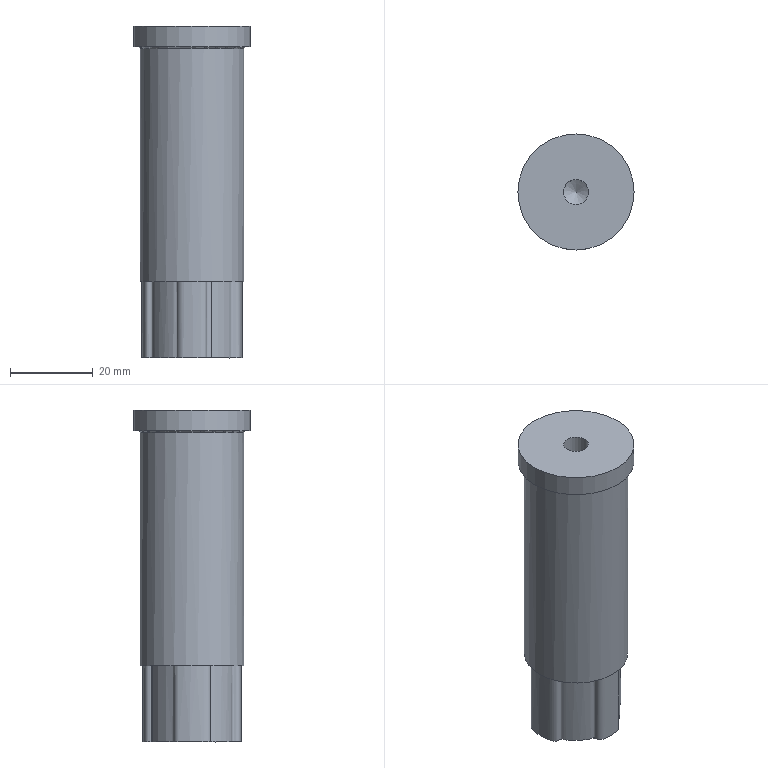Part | NX | features solid 2 | 1 solid | 12 faces | box 28 x 28 x 80 mm | volume 38145 mm3 | plane 4 | cylinder 3 | spline 3 | torus 1 | cone 1 | commonest cylinder face diameters 6 x1 25 x1 28 x1
STEP:
#1=CARTESIAN_POINT('',(12.5,-553.396,-52.641));
#2=VERTEX_POINT('',#1);
#3=CARTESIAN_POINT('',(0.,-553.396,-52.641));
#4=DIRECTION('',(0.,0.,1.));
#5=DIRECTION('',(1.,0.,0.));
#6=AXIS2_PLACEMENT_3D('',#3,#4,#5);
#7=CIRCLE('',#6,12.5);
#8=EDGE_CURVE('',#2,#2,#7,.T.);
#9=ORIENTED_EDGE('',*,*,#8,.F.);
#10=EDGE_LOOP('',(#9));
#11=FACE_BOUND('',#10,.T.);
#12=CARTESIAN_POINT('',(-4.603,-543.997,-52.641));
#13=VERTEX_POINT('',#12);
#14=CARTESIAN_POINT('',(-4.513,-543.694,-52.641));
#15=VERTEX_POINT('',#14);
#16=CARTESIAN_POINT('',(-4.513,-543.694,-52.641));
#17=CARTESIAN_POINT('',(-4.512,-543.806,-52.641));
#18=CARTESIAN_POINT('',(-4.502,-543.949,-52.641));
#19=CARTESIAN_POINT('',(-4.603,-543.997,-52.641));
#20=B_SPLINE_CURVE_WITH_KNOTS('',3,(#16,#17,#18,#19),.UNSPECIFIED.,.F.,.F.,(4,4),(0.0008113,0.001146),.UNSPECIFIED.);
#21=EDGE_CURVE('',#13,#15,#20,.F.);
#22=ORIENTED_EDGE('',*,*,#21,.F.);
#23=CARTESIAN_POINT('',(4.598,-562.799,-52.641));
#24=VERTEX_POINT('',#23);
#25=CARTESIAN_POINT('',(-4.603,-543.997,-52.641));
#26=CARTESIAN_POINT('',(-5.308,-544.333,-52.641));
#27=CARTESIAN_POINT('',(-6.291,-544.944,-52.641));
#28=CARTESIAN_POINT('',(-7.471,-545.972,-52.641));
#29=CARTESIAN_POINT('',(-8.248,-546.829,-52.641));
#30=CARTESIAN_POINT('',(-8.839,-547.592,-52.641));
#31=CARTESIAN_POINT('',(-9.219,-548.267,-52.641));
#32=CARTESIAN_POINT('',(-9.493,-548.804,-52.641));
#33=CARTESIAN_POINT('',(-10.053,-549.033,-52.641));
#34=CARTESIAN_POINT('',(-10.645,-549.002,-52.641));
#35=CARTESIAN_POINT('',(-11.186,-549.281,-52.641));
#36=CARTESIAN_POINT('',(-11.626,-549.945,-52.641));
#37=CARTESIAN_POINT('',(-11.842,-550.898,-52.641));
#38=CARTESIAN_POINT('',(-12.044,-552.036,-52.641));
#39=CARTESIAN_POINT('',(-12.119,-553.186,-52.641));
#40=CARTESIAN_POINT('',(-12.086,-554.353,-52.641));
#41=CARTESIAN_POINT('',(-11.917,-555.507,-52.641));
#42=CARTESIAN_POINT('',(-11.746,-556.471,-52.641));
#43=CARTESIAN_POINT('',(-11.428,-557.184,-52.641));
#44=CARTESIAN_POINT('',(-11.023,-557.655,-52.641));
#45=CARTESIAN_POINT('',(-10.436,-557.867,-52.641));
#46=CARTESIAN_POINT('',(-9.926,-557.72,-52.641));
#47=CARTESIAN_POINT('',(-9.524,-557.882,-52.641));
#48=CARTESIAN_POINT('',(-9.345,-558.271,-52.641));
#49=CARTESIAN_POINT('',(-9.172,-558.747,-52.641));
#50=CARTESIAN_POINT('',(-8.784,-559.217,-52.641));
#51=CARTESIAN_POINT('',(-8.338,-559.888,-52.641));
#52=CARTESIAN_POINT('',(-7.667,-560.629,-52.641));
#53=CARTESIAN_POINT('',(-6.792,-561.431,-52.641));
#54=CARTESIAN_POINT('',(-5.996,-562.048,-52.641));
#55=CARTESIAN_POINT('',(-5.292,-562.423,-52.641));
#56=CARTESIAN_POINT('',(-4.783,-562.743,-52.641));
#57=CARTESIAN_POINT('',(-4.255,-563.007,-52.641));
#58=CARTESIAN_POINT('',(-3.725,-563.027,-52.641));
#59=CARTESIAN_POINT('',(-3.437,-563.341,-52.641));
#60=CARTESIAN_POINT('',(-3.464,-563.754,-52.641));
#61=CARTESIAN_POINT('',(-3.478,-564.269,-52.641));
#62=CARTESIAN_POINT('',(-3.053,-564.739,-52.641));
#63=CARTESIAN_POINT('',(-2.367,-565.158,-52.641));
#64=CARTESIAN_POINT('',(-1.351,-565.233,-52.641));
#65=CARTESIAN_POINT('',(-0.1784,-565.334,-52.641));
#66=CARTESIAN_POINT('',(1.023,-565.285,-52.641));
#67=CARTESIAN_POINT('',(2.182,-565.183,-52.641));
#68=CARTESIAN_POINT('',(3.203,-564.762,-52.641));
#69=CARTESIAN_POINT('',(3.437,-563.977,-52.641));
#70=CARTESIAN_POINT('',(3.537,-563.131,-52.641));
#71=CARTESIAN_POINT('',(4.231,-562.959,-52.641));
#72=CARTESIAN_POINT('',(4.598,-562.799,-52.641));
#73=B_SPLINE_CURVE_WITH_KNOTS('',3,(#25,#26,#27,#28,#29,#30,#31,#32,#33,#34,#35,#36,#37,#38,#39,#40,#41,#42,#43,#44,#45,#46,#47,#48,#49,#50,#51,#52,#53,#54,#55,#56,#57,#58,#59,#60,#61,#62,#63,#64,#65,#66,#67,#68,#69,#70,#71,#72),.UNSPECIFIED.,.F.,.F.,(4,1,1,1,1,1,1,1,1,1,1,1,1,1,1,1,1,1,1,1,1,1,1,1,1,1,1,1,1,1,1,1,1,1,1,1,1,1,1,1,1,1,1,1,1,4),(0.,0.002319,0.003478,0.004637,0.005797,0.006376,0.006956,0.007536,0.008115,0.008695,0.009275,0.01043,0.01159,0.01275,0.01391,0.01507,0.01623,0.01681,0.01739,0.01797,0.01855,0.01884,0.01913,0.01971,0.02029,0.02087,0.02203,0.02319,0.02435,0.02493,0.02551,0.02608,0.02666,0.02695,0.02724,0.02782,0.0284,0.02898,0.03014,0.0313,0.03246,0.03362,0.03478,0.03536,0.03594,0.0371),.UNSPECIFIED.);
#74=EDGE_CURVE('',#13,#24,#73,.T.);
#75=ORIENTED_EDGE('',*,*,#74,.T.);
#76=CARTESIAN_POINT('',(4.598,-562.799,-52.641));
#77=CARTESIAN_POINT('',(5.32,-562.485,-52.641));
#78=CARTESIAN_POINT('',(6.283,-561.845,-52.641));
#79=CARTESIAN_POINT('',(7.451,-560.834,-52.641));
#80=CARTESIAN_POINT('',(8.122,-560.118,-52.641));
#81=CARTESIAN_POINT('',(8.588,-559.498,-52.641));
#82=CARTESIAN_POINT('',(8.952,-559.039,-52.641));
#83=CARTESIAN_POINT('',(9.211,-558.515,-52.641));
#84=CARTESIAN_POINT('',(9.494,-557.957,-52.641));
#85=CARTESIAN_POINT('',(10.094,-557.813,-52.641));
#86=CARTESIAN_POINT('',(10.882,-557.758,-52.641));
#87=CARTESIAN_POINT('',(11.636,-557.021,-52.641));
#88=CARTESIAN_POINT('',(11.837,-555.845,-52.641));
#89=CARTESIAN_POINT('',(12.046,-554.713,-52.641));
#90=CARTESIAN_POINT('',(12.11,-553.559,-52.641));
#91=CARTESIAN_POINT('',(12.074,-552.393,-52.641));
#92=CARTESIAN_POINT('',(11.9,-551.237,-52.641));
#93=CARTESIAN_POINT('',(11.733,-550.269,-52.641));
#94=CARTESIAN_POINT('',(11.396,-549.558,-52.641));
#95=CARTESIAN_POINT('',(10.959,-549.149,-52.641));
#96=CARTESIAN_POINT('',(10.397,-548.933,-52.641));
#97=CARTESIAN_POINT('',(9.901,-549.045,-52.641));
#98=CARTESIAN_POINT('',(9.507,-548.923,-52.641));
#99=CARTESIAN_POINT('',(9.314,-548.563,-52.641));
#100=CARTESIAN_POINT('',(9.187,-548.09,-52.641));
#101=CARTESIAN_POINT('',(8.819,-547.627,-52.641));
#102=CARTESIAN_POINT('',(8.359,-546.98,-52.641));
#103=CARTESIAN_POINT('',(7.72,-546.238,-52.641));
#104=CARTESIAN_POINT('',(7.018,-545.561,-52.641));
#105=CARTESIAN_POINT('',(6.391,-545.087,-52.641));
#106=CARTESIAN_POINT('',(5.923,-544.73,-52.641));
#107=CARTESIAN_POINT('',(5.411,-544.416,-52.641));
#108=CARTESIAN_POINT('',(4.843,-544.187,-52.641));
#109=CARTESIAN_POINT('',(4.466,-543.688,-52.641));
#110=CARTESIAN_POINT('',(4.464,-543.07,-52.641));
#111=CARTESIAN_POINT('',(4.266,-542.486,-52.641));
#112=CARTESIAN_POINT('',(3.618,-541.972,-52.641));
#113=CARTESIAN_POINT('',(2.628,-541.765,-52.641));
#114=CARTESIAN_POINT('',(1.466,-541.551,-52.641));
#115=CARTESIAN_POINT('',(0.2671,-541.471,-52.641));
#116=CARTESIAN_POINT('',(-0.9138,-541.495,-52.641));
#117=CARTESIAN_POINT('',(-2.087,-541.643,-52.641));
#118=CARTESIAN_POINT('',(-3.237,-541.861,-52.641));
#119=CARTESIAN_POINT('',(-4.412,-542.417,-52.641));
#120=CARTESIAN_POINT('',(-4.515,-543.293,-52.641));
#121=CARTESIAN_POINT('',(-4.513,-543.694,-52.641));
#122=B_SPLINE_CURVE_WITH_KNOTS('',3,(#76,#77,#78,#79,#80,#81,#82,#83,#84,#85,#86,#87,#88,#89,#90,#91,#92,#93,#94,#95,#96,#97,#98,#99,#100,#101,#102,#103,#104,#105,#106,#107,#108,#109,#110,#111,#112,#113,#114,#115,#116,#117,#118,#119,#120,#121),.UNSPECIFIED.,.F.,.F.,(4,1,1,1,1,1,1,1,1,1,1,1,1,1,1,1,1,1,1,1,1,1,1,1,1,1,1,1,1,1,1,1,1,1,1,1,1,1,1,1,1,1,1,4),(0.07329,0.07565,0.07683,0.07802,0.07861,0.0792,0.07979,0.08038,0.08097,0.08156,0.08274,0.08392,0.08511,0.08629,0.08747,0.08865,0.08983,0.09042,0.09101,0.0916,0.09219,0.09249,0.09279,0.09338,0.09397,0.09456,0.09574,0.09692,0.09751,0.0981,0.09869,0.09928,0.09988,0.1005,0.1011,0.1016,0.1028,0.104,0.1052,0.1064,0.1076,0.1087,0.1099,0.1111),.UNSPECIFIED.);
#123=EDGE_CURVE('',#24,#15,#122,.T.);
#124=ORIENTED_EDGE('',*,*,#123,.T.);
#125=EDGE_LOOP('',(#22,#75,#124));
#126=FACE_BOUND('',#125,.T.);
#127=CARTESIAN_POINT('',(0.,-553.396,-52.641));
#128=DIRECTION('',(0.,0.,1.));
#129=DIRECTION('',(1.,0.,0.));
#130=AXIS2_PLACEMENT_3D('',#127,#128,#129);
#131=PLANE('',#130);
#132=ADVANCED_FACE('',(#11,#126),#131,.F.);
#133=CARTESIAN_POINT('',(0.,-566.396,4.));
#134=VERTEX_POINT('',#133);
#135=CARTESIAN_POINT('',(0.,-553.396,4.));
#136=DIRECTION('',(0.,0.,-1.));
#137=DIRECTION('',(0.,-1.,0.));
#138=AXIS2_PLACEMENT_3D('',#135,#136,#137);
#139=CIRCLE('',#138,13.);
#140=EDGE_CURVE('',#134,#134,#139,.F.);
#141=ORIENTED_EDGE('',*,*,#140,.T.);
#142=EDGE_LOOP('',(#141));
#143=FACE_BOUND('',#142,.T.);
#144=CARTESIAN_POINT('',(0.,-567.396,4.));
#145=VERTEX_POINT('',#144);
#146=CARTESIAN_POINT('',(0.,-553.396,4.));
#147=DIRECTION('',(0.,0.,-1.));
#148=DIRECTION('',(0.,-1.,0.));
#149=AXIS2_PLACEMENT_3D('',#146,#147,#148);
#150=CIRCLE('',#149,14.);
#151=EDGE_CURVE('',#145,#145,#150,.T.);
#152=ORIENTED_EDGE('',*,*,#151,.T.);
#153=EDGE_LOOP('',(#152));
#154=FACE_BOUND('',#153,.T.);
#155=CARTESIAN_POINT('',(0.,-553.396,4.));
#156=DIRECTION('',(0.,0.,-1.));
#157=DIRECTION('',(0.,-1.,0.));
#158=AXIS2_PLACEMENT_3D('',#155,#156,#157);
#159=PLANE('',#158);
#160=ADVANCED_FACE('',(#143,#154),#159,.T.);
#161=ORIENTED_EDGE('',*,*,#151,.F.);
#162=EDGE_LOOP('',(#161));
#163=FACE_BOUND('',#162,.T.);
#164=CARTESIAN_POINT('',(0.,-567.396,9.));
#165=VERTEX_POINT('',#164);
#166=CARTESIAN_POINT('',(0.,-553.396,9.));
#167=DIRECTION('',(0.,0.,-1.));
#168=DIRECTION('',(0.,-1.,0.));
#169=AXIS2_PLACEMENT_3D('',#166,#167,#168);
#170=CIRCLE('',#169,14.);
#171=EDGE_CURVE('',#165,#165,#170,.T.);
#172=ORIENTED_EDGE('',*,*,#171,.T.);
#173=EDGE_LOOP('',(#172));
#174=FACE_BOUND('',#173,.T.);
#175=CARTESIAN_POINT('',(0.,-553.396,4.));
#176=DIRECTION('',(0.,0.,1.));
#177=DIRECTION('',(0.,1.,0.));
#178=AXIS2_PLACEMENT_3D('',#175,#176,#177);
#179=CYLINDRICAL_SURFACE('',#178,14.);
#180=ADVANCED_FACE('',(#163,#174),#179,.T.);
#181=CARTESIAN_POINT('',(0.,-556.396,9.));
#182=VERTEX_POINT('',#181);
#183=CARTESIAN_POINT('',(0.,-553.396,9.));
#184=DIRECTION('',(0.,0.,-1.));
#185=DIRECTION('',(0.,-1.,0.));
#186=AXIS2_PLACEMENT_3D('',#183,#184,#185);
#187=CIRCLE('',#186,3.);
#188=EDGE_CURVE('',#182,#182,#187,.T.);
#189=ORIENTED_EDGE('',*,*,#188,.T.);
#190=EDGE_LOOP('',(#189));
#191=FACE_BOUND('',#190,.T.);
#192=ORIENTED_EDGE('',*,*,#171,.F.);
#193=EDGE_LOOP('',(#192));
#194=FACE_BOUND('',#193,.T.);
#195=CARTESIAN_POINT('',(0.,-553.396,9.));
#196=DIRECTION('',(0.,0.,-1.));
#197=DIRECTION('',(0.,-1.,0.));
#198=AXIS2_PLACEMENT_3D('',#195,#196,#197);
#199=PLANE('',#198);
#200=ADVANCED_FACE('',(#191,#194),#199,.F.);
#201=CARTESIAN_POINT('',(0.,-565.896,3.5));
#202=VERTEX_POINT('',#201);
#203=CARTESIAN_POINT('',(0.,-553.396,3.5));
#204=DIRECTION('',(0.,0.,-1.));
#205=DIRECTION('',(0.,-1.,0.));
#206=AXIS2_PLACEMENT_3D('',#203,#204,#205);
#207=CIRCLE('',#206,12.5);
#208=EDGE_CURVE('',#202,#202,#207,.T.);
#209=ORIENTED_EDGE('',*,*,#208,.T.);
#210=EDGE_LOOP('',(#209));
#211=FACE_BOUND('',#210,.T.);
#212=ORIENTED_EDGE('',*,*,#8,.T.);
#213=EDGE_LOOP('',(#212));
#214=FACE_BOUND('',#213,.T.);
#215=CARTESIAN_POINT('',(0.,-553.396,-41.641));
#216=DIRECTION('',(0.,0.,1.));
#217=DIRECTION('',(0.,1.,0.));
#218=AXIS2_PLACEMENT_3D('',#215,#216,#217);
#219=CYLINDRICAL_SURFACE('',#218,12.5);
#220=ADVANCED_FACE('',(#211,#214),#219,.T.);
#221=ORIENTED_EDGE('',*,*,#208,.F.);
#222=EDGE_LOOP('',(#221));
#223=FACE_BOUND('',#222,.T.);
#224=ORIENTED_EDGE('',*,*,#140,.F.);
#225=EDGE_LOOP('',(#224));
#226=FACE_BOUND('',#225,.T.);
#227=CARTESIAN_POINT('',(0.,-553.396,3.5));
#228=DIRECTION('',(0.,0.,-1.));
#229=DIRECTION('',(0.,-1.,0.));
#230=AXIS2_PLACEMENT_3D('',#227,#228,#229);
#231=TOROIDAL_SURFACE('',#230,13.,0.5);
#232=ADVANCED_FACE('',(#223,#226),#231,.F.);
#233=CARTESIAN_POINT('',(0.,-556.396,-4.));
#234=VERTEX_POINT('',#233);
#235=CARTESIAN_POINT('',(0.,-553.396,-4.));
#236=DIRECTION('',(0.,0.,-1.));
#237=DIRECTION('',(0.,-1.,0.));
#238=AXIS2_PLACEMENT_3D('',#235,#236,#237);
#239=CIRCLE('',#238,3.);
#240=EDGE_CURVE('',#234,#234,#239,.T.);
#241=ORIENTED_EDGE('',*,*,#240,.F.);
#242=EDGE_LOOP('',(#241));
#243=FACE_BOUND('',#242,.T.);
#244=CARTESIAN_POINT('',(0.,-553.396,-5.803));
#245=VERTEX_POINT('',#244);
#246=VERTEX_LOOP('',#245);
#247=FACE_BOUND('',#246,.T.);
#248=CARTESIAN_POINT('',(0.,-553.396,-4.));
#249=DIRECTION('',(0.,0.,1.));
#250=DIRECTION('',(0.,1.,0.));
#251=AXIS2_PLACEMENT_3D('',#248,#249,#250);
#252=CONICAL_SURFACE('',#251,3.,1.03);
#253=ADVANCED_FACE('',(#243,#247),#252,.F.);
#254=ORIENTED_EDGE('',*,*,#240,.T.);
#255=EDGE_LOOP('',(#254));
#256=FACE_BOUND('',#255,.T.);
#257=ORIENTED_EDGE('',*,*,#188,.F.);
#258=EDGE_LOOP('',(#257));
#259=FACE_BOUND('',#258,.T.);
#260=CARTESIAN_POINT('',(0.,-553.396,9.));
#261=DIRECTION('',(0.,0.,-1.));
#262=DIRECTION('',(0.,-1.,0.));
#263=AXIS2_PLACEMENT_3D('',#260,#261,#262);
#264=CYLINDRICAL_SURFACE('',#263,3.);
#265=ADVANCED_FACE('',(#256,#259),#264,.F.);
#266=ORIENTED_EDGE('',*,*,#21,.T.);
#267=CARTESIAN_POINT('',(-4.513,-543.694,-71.));
#268=VERTEX_POINT('',#267);
#269=CARTESIAN_POINT('',(-4.513,-543.694,-1169.976));
#270=DIRECTION('',(0.,0.,1.));
#271=VECTOR('',#270,1000.);
#272=LINE('',#269,#271);
#273=EDGE_CURVE('',#268,#15,#272,.T.);
#274=ORIENTED_EDGE('',*,*,#273,.F.);
#275=CARTESIAN_POINT('',(-4.603,-543.997,-71.));
#276=VERTEX_POINT('',#275);
#277=CARTESIAN_POINT('',(-4.513,-543.694,-71.));
#278=CARTESIAN_POINT('',(-4.512,-543.806,-71.));
#279=CARTESIAN_POINT('',(-4.502,-543.949,-71.));
#280=CARTESIAN_POINT('',(-4.603,-543.997,-71.));
#281=B_SPLINE_CURVE_WITH_KNOTS('',3,(#277,#278,#279,#280),.UNSPECIFIED.,.F.,.F.,(4,4),(0.001516,0.001851),.UNSPECIFIED.);
#282=EDGE_CURVE('',#276,#268,#281,.F.);
#283=ORIENTED_EDGE('',*,*,#282,.F.);
#284=CARTESIAN_POINT('',(-4.603,-543.997,-1169.976));
#285=DIRECTION('',(0.,0.,1.));
#286=VECTOR('',#285,1000.);
#287=LINE('',#284,#286);
#288=EDGE_CURVE('',#276,#13,#287,.T.);
#289=ORIENTED_EDGE('',*,*,#288,.T.);
#290=EDGE_LOOP('',(#266,#274,#283,#289));
#291=FACE_BOUND('',#290,.T.);
#292=CARTESIAN_POINT('',(-4.603,-543.997,-71.));
#293=CARTESIAN_POINT('',(-4.603,-543.997,-52.641));
#294=CARTESIAN_POINT('',(-4.505,-543.951,-71.));
#295=CARTESIAN_POINT('',(-4.505,-543.951,-52.641));
#296=CARTESIAN_POINT('',(-4.512,-543.82,-71.));
#297=CARTESIAN_POINT('',(-4.512,-543.82,-52.641));
#298=CARTESIAN_POINT('',(-4.513,-543.694,-71.));
#299=CARTESIAN_POINT('',(-4.513,-543.694,-52.641));
#300=B_SPLINE_SURFACE_WITH_KNOTS('',3,1,((#292,#293),(#294,#295),(#296,#297),(#298,#299)),.SURF_OF_LINEAR_EXTRUSION.,.F.,.F.,.F.,(4,4),(2,2),(0.,1.),(0.,1.),.PIECEWISE_BEZIER_KNOTS.);
#301=ADVANCED_FACE('',(#291),#300,.F.);
#302=ORIENTED_EDGE('',*,*,#123,.F.);
#303=CARTESIAN_POINT('',(4.598,-562.799,-71.));
#304=VERTEX_POINT('',#303);
#305=CARTESIAN_POINT('',(4.598,-562.799,-1169.976));
#306=DIRECTION('',(0.,0.,1.));
#307=VECTOR('',#306,1000.);
#308=LINE('',#305,#307);
#309=EDGE_CURVE('',#304,#24,#308,.T.);
#310=ORIENTED_EDGE('',*,*,#309,.F.);
#311=CARTESIAN_POINT('',(4.598,-562.799,-71.));
#312=CARTESIAN_POINT('',(5.308,-562.49,-71.));
#313=CARTESIAN_POINT('',(6.265,-561.859,-71.));
#314=CARTESIAN_POINT('',(7.431,-560.851,-71.));
#315=CARTESIAN_POINT('',(8.088,-560.16,-71.));
#316=CARTESIAN_POINT('',(8.547,-559.55,-71.));
#317=CARTESIAN_POINT('',(8.906,-559.102,-71.));
#318=CARTESIAN_POINT('',(9.184,-558.596,-71.));
#319=CARTESIAN_POINT('',(9.423,-558.034,-71.));
#320=CARTESIAN_POINT('',(9.989,-557.814,-71.));
#321=CARTESIAN_POINT('',(10.564,-557.788,-71.));
#322=CARTESIAN_POINT('',(11.117,-557.567,-71.));
#323=CARTESIAN_POINT('',(11.612,-556.946,-71.));
#324=CARTESIAN_POINT('',(11.811,-555.988,-71.));
#325=CARTESIAN_POINT('',(12.026,-554.869,-71.));
#326=CARTESIAN_POINT('',(12.107,-553.722,-71.));
#327=CARTESIAN_POINT('',(12.085,-552.565,-71.));
#328=CARTESIAN_POINT('',(11.939,-551.423,-71.));
#329=CARTESIAN_POINT('',(11.739,-550.279,-71.));
#330=CARTESIAN_POINT('',(11.318,-549.401,-71.));
#331=CARTESIAN_POINT('',(10.627,-548.97,-71.));
#332=CARTESIAN_POINT('',(10.055,-549.011,-71.));
#333=CARTESIAN_POINT('',(9.42,-548.963,-71.));
#334=CARTESIAN_POINT('',(9.273,-548.318,-71.));
#335=CARTESIAN_POINT('',(9.,-547.827,-71.));
#336=CARTESIAN_POINT('',(8.497,-547.211,-71.));
#337=CARTESIAN_POINT('',(7.916,-546.423,-71.));
#338=CARTESIAN_POINT('',(7.077,-545.607,-71.));
#339=CARTESIAN_POINT('',(6.303,-545.014,-71.));
#340=CARTESIAN_POINT('',(5.658,-544.55,-71.));
#341=CARTESIAN_POINT('',(5.122,-544.3,-71.));
#342=CARTESIAN_POINT('',(4.573,-543.974,-71.));
#343=CARTESIAN_POINT('',(4.459,-543.327,-71.));
#344=CARTESIAN_POINT('',(4.392,-542.713,-71.));
#345=CARTESIAN_POINT('',(3.984,-542.209,-71.));
#346=CARTESIAN_POINT('',(3.412,-541.957,-71.));
#347=CARTESIAN_POINT('',(2.627,-541.759,-71.));
#348=CARTESIAN_POINT('',(1.623,-541.573,-71.));
#349=CARTESIAN_POINT('',(0.4114,-541.474,-71.));
#350=CARTESIAN_POINT('',(-0.7949,-541.487,-71.));
#351=CARTESIAN_POINT('',(-2.006,-541.626,-71.));
#352=CARTESIAN_POINT('',(-3.194,-541.853,-71.));
#353=CARTESIAN_POINT('',(-4.398,-542.386,-71.));
#354=CARTESIAN_POINT('',(-4.515,-543.284,-71.));
#355=CARTESIAN_POINT('',(-4.513,-543.694,-71.));
#356=B_SPLINE_CURVE_WITH_KNOTS('',3,(#311,#312,#313,#314,#315,#316,#317,#318,#319,#320,#321,#322,#323,#324,#325,#326,#327,#328,#329,#330,#331,#332,#333,#334,#335,#336,#337,#338,#339,#340,#341,#342,#343,#344,#345,#346,#347,#348,#349,#350,#351,#352,#353,#354,#355),.UNSPECIFIED.,.F.,.F.,(4,1,1,1,1,1,1,1,1,1,1,1,1,1,1,1,1,1,1,1,1,1,1,1,1,1,1,1,1,1,1,1,1,1,1,1,1,1,1,1,1,1,4),(0.,0.002292,0.003437,0.004583,0.005156,0.005729,0.006302,0.006875,0.007448,0.008021,0.008593,0.009166,0.01031,0.01146,0.0126,0.01375,0.0149,0.01604,0.01719,0.01776,0.01833,0.01891,0.01948,0.02005,0.02062,0.02177,0.02292,0.02406,0.02463,0.02521,0.02578,0.02635,0.02693,0.0275,0.02807,0.02864,0.02979,0.03094,0.03208,0.03323,0.03437,0.03552,0.03667),.UNSPECIFIED.);
#357=EDGE_CURVE('',#304,#268,#356,.T.);
#358=ORIENTED_EDGE('',*,*,#357,.T.);
#359=ORIENTED_EDGE('',*,*,#273,.T.);
#360=EDGE_LOOP('',(#302,#310,#358,#359));
#361=FACE_BOUND('',#360,.T.);
#362=CARTESIAN_POINT('',(4.598,-562.799,-71.));
#363=CARTESIAN_POINT('',(4.598,-562.799,-52.641));
#364=CARTESIAN_POINT('',(5.345,-562.474,-71.));
#365=CARTESIAN_POINT('',(5.345,-562.474,-52.641));
#366=CARTESIAN_POINT('',(6.317,-561.817,-71.));
#367=CARTESIAN_POINT('',(6.317,-561.817,-52.641));
#368=CARTESIAN_POINT('',(7.517,-560.781,-71.));
#369=CARTESIAN_POINT('',(7.517,-560.781,-52.641));
#370=CARTESIAN_POINT('',(8.297,-559.882,-71.));
#371=CARTESIAN_POINT('',(8.297,-559.882,-52.641));
#372=CARTESIAN_POINT('',(9.043,-559.002,-71.));
#373=CARTESIAN_POINT('',(9.043,-559.002,-52.641));
#374=CARTESIAN_POINT('',(9.466,-557.752,-71.));
#375=CARTESIAN_POINT('',(9.466,-557.752,-52.641));
#376=CARTESIAN_POINT('',(10.526,-557.859,-71.));
#377=CARTESIAN_POINT('',(10.526,-557.859,-52.641));
#378=CARTESIAN_POINT('',(11.243,-557.463,-71.));
#379=CARTESIAN_POINT('',(11.243,-557.463,-52.641));
#380=CARTESIAN_POINT('',(11.654,-556.785,-71.));
#381=CARTESIAN_POINT('',(11.654,-556.785,-52.641));
#382=CARTESIAN_POINT('',(11.853,-555.812,-71.));
#383=CARTESIAN_POINT('',(11.853,-555.812,-52.641));
#384=CARTESIAN_POINT('',(12.051,-554.657,-71.));
#385=CARTESIAN_POINT('',(12.051,-554.657,-52.641));
#386=CARTESIAN_POINT('',(12.111,-553.481,-71.));
#387=CARTESIAN_POINT('',(12.111,-553.481,-52.641));
#388=CARTESIAN_POINT('',(12.067,-552.303,-71.));
#389=CARTESIAN_POINT('',(12.067,-552.303,-52.641));
#390=CARTESIAN_POINT('',(11.878,-551.152,-71.));
#391=CARTESIAN_POINT('',(11.878,-551.152,-52.641));
#392=CARTESIAN_POINT('',(11.715,-550.156,-71.));
#393=CARTESIAN_POINT('',(11.715,-550.156,-52.641));
#394=CARTESIAN_POINT('',(11.33,-549.483,-71.));
#395=CARTESIAN_POINT('',(11.33,-549.483,-52.641));
#396=CARTESIAN_POINT('',(10.868,-549.082,-71.));
#397=CARTESIAN_POINT('',(10.868,-549.082,-52.641));
#398=CARTESIAN_POINT('',(10.28,-548.942,-71.));
#399=CARTESIAN_POINT('',(10.28,-548.942,-52.641));
#400=CARTESIAN_POINT('',(9.607,-549.074,-71.));
#401=CARTESIAN_POINT('',(9.607,-549.074,-52.641));
#402=CARTESIAN_POINT('',(9.32,-548.589,-71.));
#403=CARTESIAN_POINT('',(9.32,-548.589,-52.641));
#404=CARTESIAN_POINT('',(9.109,-547.94,-71.));
#405=CARTESIAN_POINT('',(9.109,-547.94,-52.641));
#406=CARTESIAN_POINT('',(8.732,-547.532,-71.));
#407=CARTESIAN_POINT('',(8.732,-547.532,-52.641));
#408=CARTESIAN_POINT('',(8.286,-546.861,-71.));
#409=CARTESIAN_POINT('',(8.286,-546.861,-52.641));
#410=CARTESIAN_POINT('',(7.623,-546.138,-71.));
#411=CARTESIAN_POINT('',(7.623,-546.138,-52.641));
#412=CARTESIAN_POINT('',(6.74,-545.335,-71.));
#413=CARTESIAN_POINT('',(6.74,-545.335,-52.641));
#414=CARTESIAN_POINT('',(5.972,-544.736,-71.));
#415=CARTESIAN_POINT('',(5.972,-544.736,-52.641));
#416=CARTESIAN_POINT('',(5.248,-544.35,-71.));
#417=CARTESIAN_POINT('',(5.248,-544.35,-52.641));
#418=CARTESIAN_POINT('',(4.712,-544.08,-71.));
#419=CARTESIAN_POINT('',(4.712,-544.08,-52.641));
#420=CARTESIAN_POINT('',(4.481,-543.649,-71.));
#421=CARTESIAN_POINT('',(4.481,-543.649,-52.641));
#422=CARTESIAN_POINT('',(4.457,-543.046,-71.));
#423=CARTESIAN_POINT('',(4.457,-543.046,-52.641));
#424=CARTESIAN_POINT('',(4.253,-542.47,-71.));
#425=CARTESIAN_POINT('',(4.253,-542.47,-52.641));
#426=CARTESIAN_POINT('',(3.616,-541.976,-71.));
#427=CARTESIAN_POINT('',(3.616,-541.976,-52.641));
#428=CARTESIAN_POINT('',(2.629,-541.763,-71.));
#429=CARTESIAN_POINT('',(2.629,-541.763,-52.641));
#430=CARTESIAN_POINT('',(1.46,-541.551,-71.));
#431=CARTESIAN_POINT('',(1.46,-541.551,-52.641));
#432=CARTESIAN_POINT('',(0.265,-541.471,-71.));
#433=CARTESIAN_POINT('',(0.265,-541.471,-52.641));
#434=CARTESIAN_POINT('',(-0.9301,-541.496,-71.));
#435=CARTESIAN_POINT('',(-0.9301,-541.496,-52.641));
#436=CARTESIAN_POINT('',(-2.118,-541.649,-71.));
#437=CARTESIAN_POINT('',(-2.118,-541.649,-52.641));
#438=CARTESIAN_POINT('',(-3.276,-541.869,-71.));
#439=CARTESIAN_POINT('',(-3.276,-541.869,-52.641));
#440=CARTESIAN_POINT('',(-4.421,-542.44,-71.));
#441=CARTESIAN_POINT('',(-4.421,-542.44,-52.641));
#442=CARTESIAN_POINT('',(-4.515,-543.302,-71.));
#443=CARTESIAN_POINT('',(-4.515,-543.302,-52.641));
#444=CARTESIAN_POINT('',(-4.513,-543.694,-71.));
#445=CARTESIAN_POINT('',(-4.513,-543.694,-52.641));
#446=B_SPLINE_SURFACE_WITH_KNOTS('',3,1,((#362,#363),(#364,#365),(#366,#367),(#368,#369),(#370,#371),(#372,#373),(#374,#375),(#376,#377),(#378,#379),(#380,#381),(#382,#383),(#384,#385),(#386,#387),(#388,#389),(#390,#391),(#392,#393),(#394,#395),(#396,#397),(#398,#399),(#400,#401),(#402,#403),(#404,#405),(#406,#407),(#408,#409),(#410,#411),(#412,#413),(#414,#415),(#416,#417),(#418,#419),(#420,#421),(#422,#423),(#424,#425),(#426,#427),(#428,#429),(#430,#431),(#432,#433),(#434,#435),(#436,#437),(#438,#439),(#440,#441),(#442,#443),(#444,#445)),.SURF_OF_LINEAR_EXTRUSION.,.F.,.F.,.F.,(4,1,1,1,1,1,1,1,1,1,1,1,1,1,1,1,1,1,1,1,1,1,1,1,1,1,1,1,1,1,1,1,1,1,1,1,1,1,1,4),(2,2),(0.,0.0625,0.09375,0.125,0.1562,0.1875,0.2188,0.2344,0.25,0.2812,0.3125,0.3438,0.375,0.4062,0.4375,0.4531,0.4688,0.4844,0.5,0.5156,0.5312,0.5469,0.5625,0.5938,0.625,0.6562,0.6719,0.6875,0.7031,0.7188,0.7344,0.75,0.7812,0.8125,0.8438,0.875,0.9062,0.9375,0.9688,1.),(0.,1.),.UNSPECIFIED.);
#447=ADVANCED_FACE('',(#361),#446,.T.);
#448=ORIENTED_EDGE('',*,*,#74,.F.);
#449=ORIENTED_EDGE('',*,*,#288,.F.);
#450=CARTESIAN_POINT('',(-4.603,-543.997,-71.));
#451=CARTESIAN_POINT('',(-5.317,-544.337,-71.));
#452=CARTESIAN_POINT('',(-6.314,-544.958,-71.));
#453=CARTESIAN_POINT('',(-7.518,-546.016,-71.));
#454=CARTESIAN_POINT('',(-8.31,-546.908,-71.));
#455=CARTESIAN_POINT('',(-8.916,-547.697,-71.));
#456=CARTESIAN_POINT('',(-9.278,-548.403,-71.));
#457=CARTESIAN_POINT('',(-9.74,-549.104,-71.));
#458=CARTESIAN_POINT('',(-10.928,-548.881,-71.));
#459=CARTESIAN_POINT('',(-11.664,-549.957,-71.));
#460=CARTESIAN_POINT('',(-11.878,-551.107,-71.));
#461=CARTESIAN_POINT('',(-12.071,-552.264,-71.));
#462=CARTESIAN_POINT('',(-12.121,-553.447,-71.));
#463=CARTESIAN_POINT('',(-12.064,-554.619,-71.));
#464=CARTESIAN_POINT('',(-11.856,-555.786,-71.));
#465=CARTESIAN_POINT('',(-11.65,-556.93,-71.));
#466=CARTESIAN_POINT('',(-10.958,-557.815,-71.));
#467=CARTESIAN_POINT('',(-10.162,-557.791,-71.));
#468=CARTESIAN_POINT('',(-9.499,-557.771,-71.));
#469=CARTESIAN_POINT('',(-9.317,-558.429,-71.));
#470=CARTESIAN_POINT('',(-9.032,-558.924,-71.));
#471=CARTESIAN_POINT('',(-8.668,-559.385,-71.));
#472=CARTESIAN_POINT('',(-8.23,-560.027,-71.));
#473=CARTESIAN_POINT('',(-7.557,-560.739,-71.));
#474=CARTESIAN_POINT('',(-6.684,-561.515,-71.));
#475=CARTESIAN_POINT('',(-5.903,-562.109,-71.));
#476=CARTESIAN_POINT('',(-5.214,-562.462,-71.));
#477=CARTESIAN_POINT('',(-4.727,-562.784,-71.));
#478=CARTESIAN_POINT('',(-4.199,-563.015,-71.));
#479=CARTESIAN_POINT('',(-3.638,-563.045,-71.));
#480=CARTESIAN_POINT('',(-3.431,-563.415,-71.));
#481=CARTESIAN_POINT('',(-3.476,-563.82,-71.));
#482=CARTESIAN_POINT('',(-3.446,-564.337,-71.));
#483=CARTESIAN_POINT('',(-2.997,-564.781,-71.));
#484=CARTESIAN_POINT('',(-2.301,-565.174,-71.));
#485=CARTESIAN_POINT('',(-1.291,-565.238,-71.));
#486=CARTESIAN_POINT('',(-0.1199,-565.334,-71.));
#487=CARTESIAN_POINT('',(1.065,-565.282,-71.));
#488=CARTESIAN_POINT('',(2.225,-565.176,-71.));
#489=CARTESIAN_POINT('',(3.22,-564.741,-71.));
#490=CARTESIAN_POINT('',(3.437,-563.961,-71.));
#491=CARTESIAN_POINT('',(3.546,-563.125,-71.));
#492=CARTESIAN_POINT('',(4.235,-562.957,-71.));
#493=CARTESIAN_POINT('',(4.598,-562.799,-71.));
#494=B_SPLINE_CURVE_WITH_KNOTS('',3,(#450,#451,#452,#453,#454,#455,#456,#457,#458,#459,#460,#461,#462,#463,#464,#465,#466,#467,#468,#469,#470,#471,#472,#473,#474,#475,#476,#477,#478,#479,#480,#481,#482,#483,#484,#485,#486,#487,#488,#489,#490,#491,#492,#493),.UNSPECIFIED.,.F.,.F.,(4,1,1,1,1,1,1,1,1,1,1,1,1,1,1,1,1,1,1,1,1,1,1,1,1,1,1,1,1,1,1,1,1,1,1,1,1,1,1,1,1,4),(0.07439,0.07676,0.07795,0.07913,0.08032,0.08091,0.0815,0.08269,0.08388,0.08506,0.08625,0.08744,0.08862,0.08981,0.091,0.09218,0.09277,0.09337,0.09396,0.09455,0.09515,0.09574,0.09693,0.09811,0.0993,0.09989,0.1005,0.1011,0.1017,0.102,0.1023,0.1029,0.1035,0.104,0.1052,0.1064,0.1076,0.1088,0.11,0.1106,0.1112,0.1123),.UNSPECIFIED.);
#495=EDGE_CURVE('',#276,#304,#494,.T.);
#496=ORIENTED_EDGE('',*,*,#495,.T.);
#497=ORIENTED_EDGE('',*,*,#309,.T.);
#498=EDGE_LOOP('',(#448,#449,#496,#497));
#499=FACE_BOUND('',#498,.T.);
#500=CARTESIAN_POINT('',(-4.603,-543.997,-71.));
#501=CARTESIAN_POINT('',(-4.603,-543.997,-52.641));
#502=CARTESIAN_POINT('',(-5.323,-544.339,-71.));
#503=CARTESIAN_POINT('',(-5.323,-544.339,-52.641));
#504=CARTESIAN_POINT('',(-6.339,-544.977,-71.));
#505=CARTESIAN_POINT('',(-6.339,-544.977,-52.641));
#506=CARTESIAN_POINT('',(-7.531,-546.028,-71.));
#507=CARTESIAN_POINT('',(-7.531,-546.028,-52.641));
#508=CARTESIAN_POINT('',(-8.319,-546.926,-71.));
#509=CARTESIAN_POINT('',(-8.319,-546.926,-52.641));
#510=CARTESIAN_POINT('',(-9.045,-547.842,-71.));
#511=CARTESIAN_POINT('',(-9.045,-547.842,-52.641));
#512=CARTESIAN_POINT('',(-9.435,-548.839,-71.));
#513=CARTESIAN_POINT('',(-9.435,-548.839,-52.641));
#514=CARTESIAN_POINT('',(-10.107,-549.02,-71.));
#515=CARTESIAN_POINT('',(-10.107,-549.02,-52.641));
#516=CARTESIAN_POINT('',(-10.985,-549.024,-71.));
#517=CARTESIAN_POINT('',(-10.985,-549.024,-52.641));
#518=CARTESIAN_POINT('',(-11.638,-549.871,-71.));
#519=CARTESIAN_POINT('',(-11.638,-549.871,-52.641));
#520=CARTESIAN_POINT('',(-11.864,-551.034,-71.));
#521=CARTESIAN_POINT('',(-11.864,-551.034,-52.641));
#522=CARTESIAN_POINT('',(-12.064,-552.196,-71.));
#523=CARTESIAN_POINT('',(-12.064,-552.196,-52.641));
#524=CARTESIAN_POINT('',(-12.122,-553.377,-71.));
#525=CARTESIAN_POINT('',(-12.122,-553.377,-52.641));
#526=CARTESIAN_POINT('',(-12.07,-554.559,-71.));
#527=CARTESIAN_POINT('',(-12.07,-554.559,-52.641));
#528=CARTESIAN_POINT('',(-11.871,-555.713,-71.));
#529=CARTESIAN_POINT('',(-11.871,-555.713,-52.641));
#530=CARTESIAN_POINT('',(-11.697,-556.707,-71.));
#531=CARTESIAN_POINT('',(-11.697,-556.707,-52.641));
#532=CARTESIAN_POINT('',(-11.281,-557.375,-71.));
#533=CARTESIAN_POINT('',(-11.281,-557.375,-52.641));
#534=CARTESIAN_POINT('',(-10.831,-557.794,-71.));
#535=CARTESIAN_POINT('',(-10.831,-557.794,-52.641));
#536=CARTESIAN_POINT('',(-10.171,-557.805,-71.));
#537=CARTESIAN_POINT('',(-10.171,-557.805,-52.641));
#538=CARTESIAN_POINT('',(-9.546,-557.744,-71.));
#539=CARTESIAN_POINT('',(-9.546,-557.744,-52.641));
#540=CARTESIAN_POINT('',(-9.333,-558.357,-71.));
#541=CARTESIAN_POINT('',(-9.333,-558.357,-52.641));
#542=CARTESIAN_POINT('',(-9.056,-558.904,-71.));
#543=CARTESIAN_POINT('',(-9.056,-558.904,-52.641));
#544=CARTESIAN_POINT('',(-8.694,-559.344,-71.));
#545=CARTESIAN_POINT('',(-8.694,-559.344,-52.641));
#546=CARTESIAN_POINT('',(-8.242,-560.015,-71.));
#547=CARTESIAN_POINT('',(-8.242,-560.015,-52.641));
#548=CARTESIAN_POINT('',(-7.567,-560.73,-71.));
#549=CARTESIAN_POINT('',(-7.567,-560.73,-52.641));
#550=CARTESIAN_POINT('',(-6.671,-561.525,-71.));
#551=CARTESIAN_POINT('',(-6.671,-561.525,-52.641));
#552=CARTESIAN_POINT('',(-5.89,-562.121,-71.));
#553=CARTESIAN_POINT('',(-5.89,-562.121,-52.641));
#554=CARTESIAN_POINT('',(-5.154,-562.491,-71.));
#555=CARTESIAN_POINT('',(-5.154,-562.491,-52.641));
#556=CARTESIAN_POINT('',(-4.698,-562.816,-71.));
#557=CARTESIAN_POINT('',(-4.698,-562.816,-52.641));
#558=CARTESIAN_POINT('',(-4.089,-563.017,-71.));
#559=CARTESIAN_POINT('',(-4.089,-563.017,-52.641));
#560=CARTESIAN_POINT('',(-3.414,-563.147,-71.));
#561=CARTESIAN_POINT('',(-3.414,-563.147,-52.641));
#562=CARTESIAN_POINT('',(-3.486,-563.777,-71.));
#563=CARTESIAN_POINT('',(-3.486,-563.777,-52.641));
#564=CARTESIAN_POINT('',(-3.41,-564.406,-71.));
#565=CARTESIAN_POINT('',(-3.41,-564.406,-52.641));
#566=CARTESIAN_POINT('',(-2.94,-564.819,-71.));
#567=CARTESIAN_POINT('',(-2.94,-564.819,-52.641));
#568=CARTESIAN_POINT('',(-2.247,-565.184,-71.));
#569=CARTESIAN_POINT('',(-2.247,-565.184,-52.641));
#570=CARTESIAN_POINT('',(-1.214,-565.247,-71.));
#571=CARTESIAN_POINT('',(-1.214,-565.247,-52.641));
#572=CARTESIAN_POINT('',(-0.03182,-565.335,-71.));
#573=CARTESIAN_POINT('',(-0.03182,-565.335,-52.641));
#574=CARTESIAN_POINT('',(1.174,-565.273,-71.));
#575=CARTESIAN_POINT('',(1.174,-565.273,-52.641));
#576=CARTESIAN_POINT('',(2.359,-565.162,-71.));
#577=CARTESIAN_POINT('',(2.359,-565.162,-52.641));
#578=CARTESIAN_POINT('',(3.494,-564.523,-71.));
#579=CARTESIAN_POINT('',(3.494,-564.523,-52.641));
#580=CARTESIAN_POINT('',(3.398,-563.154,-71.));
#581=CARTESIAN_POINT('',(3.398,-563.154,-52.641));
#582=CARTESIAN_POINT('',(4.223,-562.962,-71.));
#583=CARTESIAN_POINT('',(4.223,-562.962,-52.641));
#584=CARTESIAN_POINT('',(4.598,-562.799,-71.));
#585=CARTESIAN_POINT('',(4.598,-562.799,-52.641));
#586=B_SPLINE_SURFACE_WITH_KNOTS('',3,1,((#500,#501),(#502,#503),(#504,#505),(#506,#507),(#508,#509),(#510,#511),(#512,#513),(#514,#515),(#516,#517),(#518,#519),(#520,#521),(#522,#523),(#524,#525),(#526,#527),(#528,#529),(#530,#531),(#532,#533),(#534,#535),(#536,#537),(#538,#539),(#540,#541),(#542,#543),(#544,#545),(#546,#547),(#548,#549),(#550,#551),(#552,#553),(#554,#555),(#556,#557),(#558,#559),(#560,#561),(#562,#563),(#564,#565),(#566,#567),(#568,#569),(#570,#571),(#572,#573),(#574,#575),(#576,#577),(#578,#579),(#580,#581),(#582,#583),(#584,#585)),.SURF_OF_LINEAR_EXTRUSION.,.F.,.F.,.F.,(4,1,1,1,1,1,1,1,1,1,1,1,1,1,1,1,1,1,1,1,1,1,1,1,1,1,1,1,1,1,1,1,1,1,1,1,1,1,1,1,4),(2,2),(0.,0.0625,0.09375,0.125,0.1562,0.1875,0.2031,0.2188,0.25,0.2812,0.3125,0.3438,0.375,0.4062,0.4375,0.4531,0.4688,0.4844,0.5,0.5156,0.5312,0.5469,0.5625,0.5938,0.625,0.6562,0.6719,0.6875,0.7031,0.7188,0.7344,0.75,0.7656,0.7812,0.8125,0.8438,0.875,0.9062,0.9375,0.9688,1.),(0.,1.),.UNSPECIFIED.);
#587=ADVANCED_FACE('',(#499),#586,.T.);
#588=ORIENTED_EDGE('',*,*,#282,.T.);
#589=ORIENTED_EDGE('',*,*,#357,.F.);
#590=ORIENTED_EDGE('',*,*,#495,.F.);
#591=EDGE_LOOP('',(#588,#589,#590));
#592=FACE_BOUND('',#591,.T.);
#593=CARTESIAN_POINT('',(0.,-543.896,-71.));
#594=DIRECTION('',(0.,0.,1.));
#595=DIRECTION('',(0.,1.,0.));
#596=AXIS2_PLACEMENT_3D('',#593,#594,#595);
#597=PLANE('',#596);
#598=ADVANCED_FACE('',(#592),#597,.F.);
#599=CLOSED_SHELL('',(#132,#160,#180,#200,#220,#232,#253,#265,#301,#447,#587,#598));
#600=MANIFOLD_SOLID_BREP('',#599);
#601=(LENGTH_UNIT()NAMED_UNIT(*)SI_UNIT(.MILLI.,.METRE.));
#602=UNCERTAINTY_MEASURE_WITH_UNIT(LENGTH_MEASURE(0.0508),#601,'','');
#603=(NAMED_UNIT(*)PLANE_ANGLE_UNIT()SI_UNIT($,.RADIAN.));
#604=(NAMED_UNIT(*)SI_UNIT($,.STERADIAN.)SOLID_ANGLE_UNIT());
#605=(GEOMETRIC_REPRESENTATION_CONTEXT(3)GLOBAL_UNCERTAINTY_ASSIGNED_CONTEXT((#602))GLOBAL_UNIT_ASSIGNED_CONTEXT((#601,#603,#604))REPRESENTATION_CONTEXT('',''));
#606=ADVANCED_BREP_SHAPE_REPRESENTATION('',(#600),#605);